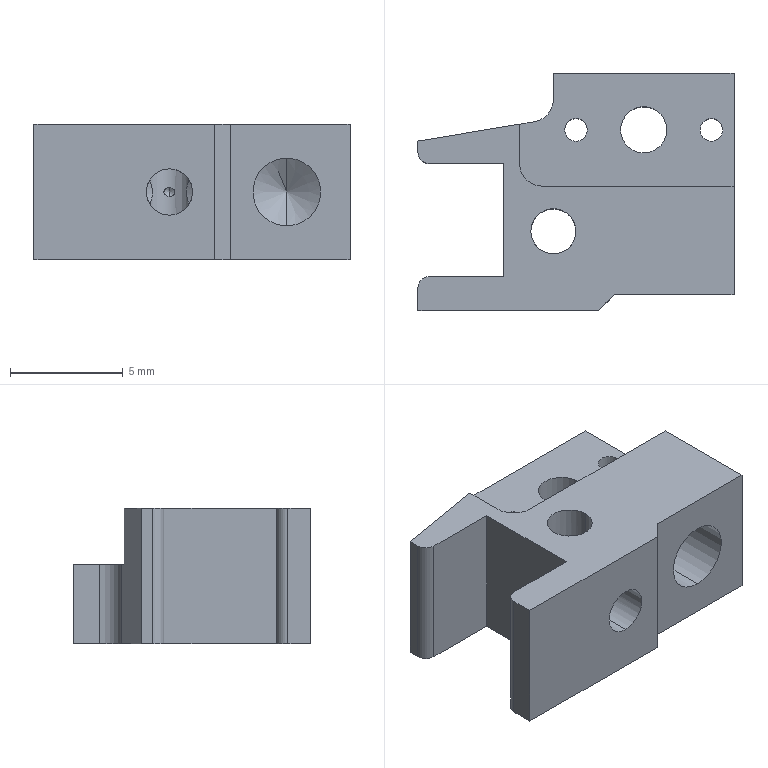Part | SolidWorks | features HoleWzd 5, ICE 4, Fillet 2, Extrusion 1 | 1 solid | 40 faces | box 14 x 10.5 x 6 mm | volume 468.744 mm3 | cylinder 17 | plane 17 | cone 6 | commonest cylinder face diameters 1 x6 2 x5 2.05 x4 3 x2
STEP:
#1=CARTESIAN_POINT('',(-1.,-2.75,1.025));
#2=VERTEX_POINT('',#1);
#3=CARTESIAN_POINT('',(-2.,-1.75,0.225));
#4=VERTEX_POINT('',#3);
#5=CARTESIAN_POINT('',(-1.,-2.75,1.025));
#6=CARTESIAN_POINT('',(-1.149,-2.75,1.025));
#7=CARTESIAN_POINT('',(-1.299,-2.714,0.9901));
#8=CARTESIAN_POINT('',(-1.55,-2.597,0.876));
#9=CARTESIAN_POINT('',(-1.654,-2.516,0.7982));
#10=CARTESIAN_POINT('',(-1.82,-2.336,0.6269));
#11=CARTESIAN_POINT('',(-1.882,-2.236,0.5323));
#12=CARTESIAN_POINT('',(-1.948,-2.074,0.3934));
#13=CARTESIAN_POINT('',(-1.966,-2.018,0.3467));
#14=CARTESIAN_POINT('',(-1.985,-1.925,0.2844));
#15=CARTESIAN_POINT('',(-1.99,-1.893,0.265));
#16=CARTESIAN_POINT('',(-1.998,-1.825,0.235));
#17=CARTESIAN_POINT('',(-2.,-1.787,0.225));
#18=CARTESIAN_POINT('',(-2.,-1.75,0.225));
#19=B_SPLINE_CURVE_WITH_KNOTS('',3,(#5,#6,#7,#8,#9,#10,#11,#12,#13,#14,#15,#16,#17,#18),.UNSPECIFIED.,.F.,.F.,(4,2,2,2,2,2,4),(0.002424,0.002875,0.003325,0.003776,0.004001,0.004114,0.004226),.UNSPECIFIED.);
#20=EDGE_CURVE('',#2,#4,#19,.T.);
#21=ORIENTED_EDGE('',*,*,#20,.F.);
#22=CARTESIAN_POINT('',(-1.,-5.25,1.025));
#23=VERTEX_POINT('',#22);
#24=CARTESIAN_POINT('',(-1.,-5.25,1.025));
#25=DIRECTION('',(0.,-1.,0.));
#26=VECTOR('',#25,1000.);
#27=LINE('',#24,#26);
#28=EDGE_CURVE('',#2,#23,#27,.T.);
#29=ORIENTED_EDGE('',*,*,#28,.T.);
#30=CARTESIAN_POINT('',(-1.,-5.25,-1.025));
#31=VERTEX_POINT('',#30);
#32=CARTESIAN_POINT('',(-1.,-5.25,0.));
#33=DIRECTION('',(0.,-1.,0.));
#34=DIRECTION('',(0.,0.,-1.));
#35=AXIS2_PLACEMENT_3D('',#32,#33,#34);
#36=CIRCLE('',#35,1.025);
#37=EDGE_CURVE('',#23,#31,#36,.T.);
#38=ORIENTED_EDGE('',*,*,#37,.T.);
#39=CARTESIAN_POINT('',(-1.,-2.75,-1.025));
#40=VERTEX_POINT('',#39);
#41=CARTESIAN_POINT('',(-1.,-5.25,-1.025));
#42=DIRECTION('',(0.,-1.,0.));
#43=VECTOR('',#42,1000.);
#44=LINE('',#41,#43);
#45=EDGE_CURVE('',#40,#31,#44,.T.);
#46=ORIENTED_EDGE('',*,*,#45,.F.);
#47=CARTESIAN_POINT('',(-2.,-1.75,-0.225));
#48=VERTEX_POINT('',#47);
#49=CARTESIAN_POINT('',(-2.,-1.75,-0.225));
#50=CARTESIAN_POINT('',(-2.,-1.825,-0.225));
#51=CARTESIAN_POINT('',(-1.991,-1.895,-0.2639));
#52=CARTESIAN_POINT('',(-1.966,-2.018,-0.3468));
#53=CARTESIAN_POINT('',(-1.948,-2.074,-0.3932));
#54=CARTESIAN_POINT('',(-1.882,-2.236,-0.5328));
#55=CARTESIAN_POINT('',(-1.819,-2.336,-0.6275));
#56=CARTESIAN_POINT('',(-1.654,-2.517,-0.7983));
#57=CARTESIAN_POINT('',(-1.55,-2.597,-0.876));
#58=CARTESIAN_POINT('',(-1.36,-2.686,-0.9622));
#59=CARTESIAN_POINT('',(-1.293,-2.709,-0.985));
#60=CARTESIAN_POINT('',(-1.15,-2.741,-1.017));
#61=CARTESIAN_POINT('',(-1.075,-2.75,-1.025));
#62=CARTESIAN_POINT('',(-1.,-2.75,-1.025));
#63=B_SPLINE_CURVE_WITH_KNOTS('',3,(#49,#50,#51,#52,#53,#54,#55,#56,#57,#58,#59,#60,#61,#62),.UNSPECIFIED.,.F.,.F.,(4,2,2,2,2,2,4),(0.0006218,0.0008471,0.001072,0.001523,0.001974,0.002199,0.002424),.UNSPECIFIED.);
#64=EDGE_CURVE('',#48,#40,#63,.T.);
#65=ORIENTED_EDGE('',*,*,#64,.F.);
#66=CARTESIAN_POINT('',(-1.866,-1.25,-0.5483));
#67=VERTEX_POINT('',#66);
#68=CARTESIAN_POINT('',(-1.866,-1.25,-0.5483));
#69=CARTESIAN_POINT('',(-1.907,-1.321,-0.4836));
#70=CARTESIAN_POINT('',(-1.938,-1.395,-0.4176));
#71=CARTESIAN_POINT('',(-1.973,-1.515,-0.3245));
#72=CARTESIAN_POINT('',(-1.982,-1.557,-0.2942));
#73=CARTESIAN_POINT('',(-1.996,-1.647,-0.2444));
#74=CARTESIAN_POINT('',(-2.,-1.698,-0.225));
#75=CARTESIAN_POINT('',(-2.,-1.75,-0.225));
#76=B_SPLINE_CURVE_WITH_KNOTS('',3,(#68,#69,#70,#71,#72,#73,#74,#75),.UNSPECIFIED.,.F.,.F.,(4,2,2,4),(0.,0.0003109,0.0004664,0.0006218),.UNSPECIFIED.);
#77=EDGE_CURVE('',#67,#48,#76,.T.);
#78=ORIENTED_EDGE('',*,*,#77,.F.);
#79=CARTESIAN_POINT('',(-1.866,-1.25,0.5483));
#80=VERTEX_POINT('',#79);
#81=CARTESIAN_POINT('',(-1.,-1.25,0.));
#82=DIRECTION('',(0.,-1.,0.));
#83=DIRECTION('',(0.,0.,-1.));
#84=AXIS2_PLACEMENT_3D('',#81,#82,#83);
#85=CIRCLE('',#84,1.025);
#86=EDGE_CURVE('',#80,#67,#85,.T.);
#87=ORIENTED_EDGE('',*,*,#86,.F.);
#88=CARTESIAN_POINT('',(-2.,-1.75,0.225));
#89=CARTESIAN_POINT('',(-2.,-1.698,0.225));
#90=CARTESIAN_POINT('',(-1.996,-1.647,0.2444));
#91=CARTESIAN_POINT('',(-1.982,-1.556,0.2945));
#92=CARTESIAN_POINT('',(-1.973,-1.515,0.3244));
#93=CARTESIAN_POINT('',(-1.939,-1.395,0.4171));
#94=CARTESIAN_POINT('',(-1.907,-1.321,0.4837));
#95=CARTESIAN_POINT('',(-1.866,-1.25,0.5483));
#96=B_SPLINE_CURVE_WITH_KNOTS('',3,(#88,#89,#90,#91,#92,#93,#94,#95),.UNSPECIFIED.,.F.,.F.,(4,2,2,4),(0.004226,0.004383,0.00454,0.004853),.UNSPECIFIED.);
#97=EDGE_CURVE('',#4,#80,#96,.T.);
#98=ORIENTED_EDGE('',*,*,#97,.F.);
#99=EDGE_LOOP('',(#21,#29,#38,#46,#65,#78,#87,#98));
#100=FACE_OUTER_BOUND('',#99,.T.);
#101=CARTESIAN_POINT('',(-1.,-5.25,0.));
#102=DIRECTION('',(0.,-1.,0.));
#103=DIRECTION('',(0.,0.,-1.));
#104=AXIS2_PLACEMENT_3D('',#101,#102,#103);
#105=CYLINDRICAL_SURFACE('',#104,1.025);
#106=ADVANCED_FACE('',(#100),#105,.F.);
#107=CARTESIAN_POINT('',(-1.,-0.6341,0.));
#108=VERTEX_POINT('',#107);
#109=CARTESIAN_POINT('',(-1.,-0.75,-0.1929));
#110=VERTEX_POINT('',#109);
#111=CARTESIAN_POINT('',(-1.,-1.25,-1.025));
#112=DIRECTION('',(0.,-0.515,-0.8572));
#113=VECTOR('',#112,1000.);
#114=LINE('',#111,#113);
#115=EDGE_CURVE('',#108,#110,#114,.T.);
#116=ORIENTED_EDGE('',*,*,#115,.F.);
#117=CARTESIAN_POINT('',(-1.,-0.75,0.1929));
#118=VERTEX_POINT('',#117);
#119=CARTESIAN_POINT('',(-1.,-1.25,1.025));
#120=DIRECTION('',(0.,-0.515,0.8572));
#121=VECTOR('',#120,1000.);
#122=LINE('',#119,#121);
#123=EDGE_CURVE('',#108,#118,#122,.T.);
#124=ORIENTED_EDGE('',*,*,#123,.T.);
#125=CARTESIAN_POINT('',(-1.,-0.75,-0.1929));
#126=CARTESIAN_POINT('',(-1.057,-0.75,-0.1929));
#127=CARTESIAN_POINT('',(-1.114,-0.7554,-0.1757));
#128=CARTESIAN_POINT('',(-1.207,-0.7704,-0.1091));
#129=CARTESIAN_POINT('',(-1.243,-0.7799,-0.05678));
#130=CARTESIAN_POINT('',(-1.243,-0.7799,0.02858));
#131=CARTESIAN_POINT('',(-1.233,-0.7775,0.0572));
#132=CARTESIAN_POINT('',(-1.203,-0.7708,0.1054));
#133=CARTESIAN_POINT('',(-1.183,-0.7666,0.126));
#134=CARTESIAN_POINT('',(-1.114,-0.7555,0.1753));
#135=CARTESIAN_POINT('',(-1.057,-0.75,0.1929));
#136=CARTESIAN_POINT('',(-1.,-0.75,0.1929));
#137=B_SPLINE_CURVE_WITH_KNOTS('',3,(#125,#126,#127,#128,#129,#130,#131,#132,#133,#134,#135,#136),.UNSPECIFIED.,.F.,.F.,(4,2,2,2,2,4),(0.001171,0.001342,0.001513,0.001599,0.001685,0.001856),.UNSPECIFIED.);
#138=EDGE_CURVE('',#110,#118,#137,.T.);
#139=ORIENTED_EDGE('',*,*,#138,.F.);
#140=EDGE_LOOP('',(#116,#124,#139));
#141=FACE_OUTER_BOUND('',#140,.T.);
#142=CARTESIAN_POINT('',(-1.,-1.25,0.));
#143=DIRECTION('',(0.,-1.,0.));
#144=DIRECTION('',(0.,0.,-1.));
#145=AXIS2_PLACEMENT_3D('',#142,#143,#144);
#146=CONICAL_SURFACE('',#145,1.025,1.03);
#147=ADVANCED_FACE('',(#141),#146,.F.);
#148=CARTESIAN_POINT('',(4.2,-0.55,1.5));
#149=VERTEX_POINT('',#148);
#150=CARTESIAN_POINT('',(4.2,-0.55,-1.5));
#151=VERTEX_POINT('',#150);
#152=CARTESIAN_POINT('',(4.2,-0.55,0.));
#153=DIRECTION('',(0.,-1.,0.));
#154=DIRECTION('',(0.,0.,-1.));
#155=AXIS2_PLACEMENT_3D('',#152,#153,#154);
#156=CIRCLE('',#155,1.5);
#157=EDGE_CURVE('',#149,#151,#156,.T.);
#158=ORIENTED_EDGE('',*,*,#157,.F.);
#159=CARTESIAN_POINT('',(4.2,-4.55,1.5));
#160=VERTEX_POINT('',#159);
#161=CARTESIAN_POINT('',(4.2,-4.55,1.5));
#162=DIRECTION('',(0.,-1.,0.));
#163=VECTOR('',#162,1000.);
#164=LINE('',#161,#163);
#165=EDGE_CURVE('',#149,#160,#164,.T.);
#166=ORIENTED_EDGE('',*,*,#165,.T.);
#167=CARTESIAN_POINT('',(4.2,-4.55,-1.5));
#168=VERTEX_POINT('',#167);
#169=CARTESIAN_POINT('',(4.2,-4.55,0.));
#170=DIRECTION('',(0.,-1.,0.));
#171=DIRECTION('',(0.,0.,-1.));
#172=AXIS2_PLACEMENT_3D('',#169,#170,#171);
#173=CIRCLE('',#172,1.5);
#174=EDGE_CURVE('',#160,#168,#173,.T.);
#175=ORIENTED_EDGE('',*,*,#174,.T.);
#176=CARTESIAN_POINT('',(4.2,-4.55,-1.5));
#177=DIRECTION('',(0.,-1.,0.));
#178=VECTOR('',#177,1000.);
#179=LINE('',#176,#178);
#180=EDGE_CURVE('',#151,#168,#179,.T.);
#181=ORIENTED_EDGE('',*,*,#180,.F.);
#182=EDGE_LOOP('',(#158,#166,#175,#181));
#183=FACE_OUTER_BOUND('',#182,.T.);
#184=CARTESIAN_POINT('',(4.2,-4.55,0.));
#185=DIRECTION('',(0.,-1.,0.));
#186=DIRECTION('',(0.,0.,-1.));
#187=AXIS2_PLACEMENT_3D('',#184,#185,#186);
#188=CYLINDRICAL_SURFACE('',#187,1.5);
#189=ADVANCED_FACE('',(#183),#188,.F.);
#190=CARTESIAN_POINT('',(4.2,0.3513,0.));
#191=VERTEX_POINT('',#190);
#192=CARTESIAN_POINT('',(4.2,-0.55,-1.5));
#193=DIRECTION('',(0.,-0.515,-0.8572));
#194=VECTOR('',#193,1000.);
#195=LINE('',#192,#194);
#196=EDGE_CURVE('',#191,#151,#195,.T.);
#197=ORIENTED_EDGE('',*,*,#196,.F.);
#198=CARTESIAN_POINT('',(4.2,-0.55,1.5));
#199=DIRECTION('',(0.,-0.515,0.8572));
#200=VECTOR('',#199,1000.);
#201=LINE('',#198,#200);
#202=EDGE_CURVE('',#191,#149,#201,.T.);
#203=ORIENTED_EDGE('',*,*,#202,.T.);
#204=ORIENTED_EDGE('',*,*,#157,.T.);
#205=EDGE_LOOP('',(#197,#203,#204));
#206=FACE_OUTER_BOUND('',#205,.T.);
#207=CARTESIAN_POINT('',(4.2,-0.55,0.));
#208=DIRECTION('',(0.,-1.,0.));
#209=DIRECTION('',(0.,0.,-1.));
#210=AXIS2_PLACEMENT_3D('',#207,#208,#209);
#211=CONICAL_SURFACE('',#210,1.5,1.03);
#212=ADVANCED_FACE('',(#206),#211,.F.);
#213=CARTESIAN_POINT('',(-2.,-1.75,-3.));
#214=VERTEX_POINT('',#213);
#215=CARTESIAN_POINT('',(0.,-1.75,-3.));
#216=VERTEX_POINT('',#215);
#217=CARTESIAN_POINT('',(-1.,-1.75,-3.));
#218=DIRECTION('',(0.,0.,1.));
#219=DIRECTION('',(1.,0.,0.));
#220=AXIS2_PLACEMENT_3D('',#217,#218,#219);
#221=CIRCLE('',#220,1.);
#222=EDGE_CURVE('',#214,#216,#221,.T.);
#223=ORIENTED_EDGE('',*,*,#222,.F.);
#224=CARTESIAN_POINT('',(-2.,-1.75,3.));
#225=DIRECTION('',(0.,0.,1.));
#226=VECTOR('',#225,1000.);
#227=LINE('',#224,#226);
#228=EDGE_CURVE('',#214,#48,#227,.T.);
#229=ORIENTED_EDGE('',*,*,#228,.T.);
#230=ORIENTED_EDGE('',*,*,#64,.T.);
#231=CARTESIAN_POINT('',(0.,-1.75,-0.225));
#232=VERTEX_POINT('',#231);
#233=CARTESIAN_POINT('',(-1.,-2.75,-1.025));
#234=CARTESIAN_POINT('',(-0.8509,-2.75,-1.025));
#235=CARTESIAN_POINT('',(-0.7012,-2.714,-0.9901));
#236=CARTESIAN_POINT('',(-0.4503,-2.597,-0.876));
#237=CARTESIAN_POINT('',(-0.346,-2.516,-0.7982));
#238=CARTESIAN_POINT('',(-0.1804,-2.336,-0.6269));
#239=CARTESIAN_POINT('',(-0.1181,-2.236,-0.5323));
#240=CARTESIAN_POINT('',(-0.05212,-2.074,-0.3934));
#241=CARTESIAN_POINT('',(-0.03443,-2.018,-0.3467));
#242=CARTESIAN_POINT('',(-0.01502,-1.925,-0.2844));
#243=CARTESIAN_POINT('',(-0.009736,-1.893,-0.265));
#244=CARTESIAN_POINT('',(-0.002191,-1.825,-0.235));
#245=CARTESIAN_POINT('',(0.,-1.787,-0.225));
#246=CARTESIAN_POINT('',(0.,-1.75,-0.225));
#247=B_SPLINE_CURVE_WITH_KNOTS('',3,(#233,#234,#235,#236,#237,#238,#239,#240,#241,#242,#243,#244,#245,#246),.UNSPECIFIED.,.F.,.F.,(4,2,2,2,2,2,4),(0.002424,0.002875,0.003325,0.003776,0.004001,0.004114,0.004226),.UNSPECIFIED.);
#248=EDGE_CURVE('',#40,#232,#247,.T.);
#249=ORIENTED_EDGE('',*,*,#248,.T.);
#250=CARTESIAN_POINT('',(0.,-1.75,3.));
#251=DIRECTION('',(0.,0.,1.));
#252=VECTOR('',#251,1000.);
#253=LINE('',#250,#252);
#254=EDGE_CURVE('',#216,#232,#253,.T.);
#255=ORIENTED_EDGE('',*,*,#254,.F.);
#256=EDGE_LOOP('',(#223,#229,#230,#249,#255));
#257=FACE_OUTER_BOUND('',#256,.T.);
#258=CARTESIAN_POINT('',(-1.,-1.75,3.));
#259=DIRECTION('',(0.,0.,1.));
#260=DIRECTION('',(1.,0.,0.));
#261=AXIS2_PLACEMENT_3D('',#258,#259,#260);
#262=CYLINDRICAL_SURFACE('',#261,1.);
#263=ADVANCED_FACE('',(#257),#262,.F.);
#264=CARTESIAN_POINT('',(0.,-1.75,0.225));
#265=VERTEX_POINT('',#264);
#266=CARTESIAN_POINT('',(0.,-1.75,0.225));
#267=CARTESIAN_POINT('',(0.,-1.825,0.225));
#268=CARTESIAN_POINT('',(-0.008603,-1.895,0.2639));
#269=CARTESIAN_POINT('',(-0.03449,-2.018,0.3468));
#270=CARTESIAN_POINT('',(-0.05201,-2.074,0.3932));
#271=CARTESIAN_POINT('',(-0.1183,-2.236,0.5328));
#272=CARTESIAN_POINT('',(-0.1808,-2.336,0.6275));
#273=CARTESIAN_POINT('',(-0.3462,-2.517,0.7983));
#274=CARTESIAN_POINT('',(-0.45,-2.597,0.876));
#275=CARTESIAN_POINT('',(-0.6399,-2.686,0.9622));
#276=CARTESIAN_POINT('',(-0.7072,-2.709,0.985));
#277=CARTESIAN_POINT('',(-0.8503,-2.741,1.017));
#278=CARTESIAN_POINT('',(-0.9254,-2.75,1.025));
#279=CARTESIAN_POINT('',(-1.,-2.75,1.025));
#280=B_SPLINE_CURVE_WITH_KNOTS('',3,(#266,#267,#268,#269,#270,#271,#272,#273,#274,#275,#276,#277,#278,#279),.UNSPECIFIED.,.F.,.F.,(4,2,2,2,2,2,4),(0.0006218,0.0008471,0.001072,0.001523,0.001974,0.002199,0.002424),.UNSPECIFIED.);
#281=EDGE_CURVE('',#265,#2,#280,.T.);
#282=ORIENTED_EDGE('',*,*,#281,.T.);
#283=ORIENTED_EDGE('',*,*,#20,.T.);
#284=CARTESIAN_POINT('',(-2.,-1.75,3.));
#285=VERTEX_POINT('',#284);
#286=CARTESIAN_POINT('',(-2.,-1.75,3.));
#287=DIRECTION('',(0.,0.,1.));
#288=VECTOR('',#287,1000.);
#289=LINE('',#286,#288);
#290=EDGE_CURVE('',#4,#285,#289,.T.);
#291=ORIENTED_EDGE('',*,*,#290,.T.);
#292=CARTESIAN_POINT('',(0.,-1.75,3.));
#293=VERTEX_POINT('',#292);
#294=CARTESIAN_POINT('',(-1.,-1.75,3.));
#295=DIRECTION('',(0.,0.,1.));
#296=DIRECTION('',(1.,0.,0.));
#297=AXIS2_PLACEMENT_3D('',#294,#295,#296);
#298=CIRCLE('',#297,1.);
#299=EDGE_CURVE('',#285,#293,#298,.T.);
#300=ORIENTED_EDGE('',*,*,#299,.T.);
#301=CARTESIAN_POINT('',(0.,-1.75,3.));
#302=DIRECTION('',(0.,0.,1.));
#303=VECTOR('',#302,1000.);
#304=LINE('',#301,#303);
#305=EDGE_CURVE('',#265,#293,#304,.T.);
#306=ORIENTED_EDGE('',*,*,#305,.F.);
#307=EDGE_LOOP('',(#282,#283,#291,#300,#306));
#308=FACE_OUTER_BOUND('',#307,.T.);
#309=CARTESIAN_POINT('',(-1.,-1.75,3.));
#310=DIRECTION('',(0.,0.,1.));
#311=DIRECTION('',(1.,0.,0.));
#312=AXIS2_PLACEMENT_3D('',#309,#310,#311);
#313=CYLINDRICAL_SURFACE('',#312,1.);
#314=ADVANCED_FACE('',(#308),#313,.F.);
#315=CARTESIAN_POINT('',(-0.5,2.75,-3.));
#316=VERTEX_POINT('',#315);
#317=CARTESIAN_POINT('',(0.5,2.75,-3.));
#318=VERTEX_POINT('',#317);
#319=CARTESIAN_POINT('',(0.,2.75,-3.));
#320=DIRECTION('',(0.,0.,1.));
#321=DIRECTION('',(1.,0.,0.));
#322=AXIS2_PLACEMENT_3D('',#319,#320,#321);
#323=CIRCLE('',#322,0.5);
#324=EDGE_CURVE('',#316,#318,#323,.T.);
#325=ORIENTED_EDGE('',*,*,#324,.F.);
#326=CARTESIAN_POINT('',(-0.5,2.75,0.5));
#327=VERTEX_POINT('',#326);
#328=CARTESIAN_POINT('',(-0.5,2.75,0.5));
#329=DIRECTION('',(0.,0.,1.));
#330=VECTOR('',#329,1000.);
#331=LINE('',#328,#330);
#332=EDGE_CURVE('',#316,#327,#331,.T.);
#333=ORIENTED_EDGE('',*,*,#332,.T.);
#334=CARTESIAN_POINT('',(0.5,2.75,0.5));
#335=VERTEX_POINT('',#334);
#336=CARTESIAN_POINT('',(0.,2.75,0.5));
#337=DIRECTION('',(0.,0.,1.));
#338=DIRECTION('',(1.,0.,0.));
#339=AXIS2_PLACEMENT_3D('',#336,#337,#338);
#340=CIRCLE('',#339,0.5);
#341=EDGE_CURVE('',#327,#335,#340,.T.);
#342=ORIENTED_EDGE('',*,*,#341,.T.);
#343=CARTESIAN_POINT('',(0.5,2.75,0.5));
#344=DIRECTION('',(0.,0.,1.));
#345=VECTOR('',#344,1000.);
#346=LINE('',#343,#345);
#347=EDGE_CURVE('',#318,#335,#346,.T.);
#348=ORIENTED_EDGE('',*,*,#347,.F.);
#349=EDGE_LOOP('',(#325,#333,#342,#348));
#350=FACE_OUTER_BOUND('',#349,.T.);
#351=CARTESIAN_POINT('',(0.,2.75,0.5));
#352=DIRECTION('',(0.,0.,1.));
#353=DIRECTION('',(1.,0.,0.));
#354=AXIS2_PLACEMENT_3D('',#351,#352,#353);
#355=CYLINDRICAL_SURFACE('',#354,0.5);
#356=ADVANCED_FACE('',(#350),#355,.F.);
#357=CARTESIAN_POINT('',(5.5,2.75,-3.));
#358=VERTEX_POINT('',#357);
#359=CARTESIAN_POINT('',(6.5,2.75,-3.));
#360=VERTEX_POINT('',#359);
#361=CARTESIAN_POINT('',(6.,2.75,-3.));
#362=DIRECTION('',(0.,0.,1.));
#363=DIRECTION('',(1.,0.,0.));
#364=AXIS2_PLACEMENT_3D('',#361,#362,#363);
#365=CIRCLE('',#364,0.5);
#366=EDGE_CURVE('',#358,#360,#365,.T.);
#367=ORIENTED_EDGE('',*,*,#366,.F.);
#368=CARTESIAN_POINT('',(5.5,2.75,0.5));
#369=VERTEX_POINT('',#368);
#370=CARTESIAN_POINT('',(5.5,2.75,0.5));
#371=DIRECTION('',(0.,0.,1.));
#372=VECTOR('',#371,1000.);
#373=LINE('',#370,#372);
#374=EDGE_CURVE('',#358,#369,#373,.T.);
#375=ORIENTED_EDGE('',*,*,#374,.T.);
#376=CARTESIAN_POINT('',(6.5,2.75,0.5));
#377=VERTEX_POINT('',#376);
#378=CARTESIAN_POINT('',(6.,2.75,0.5));
#379=DIRECTION('',(0.,0.,1.));
#380=DIRECTION('',(1.,0.,0.));
#381=AXIS2_PLACEMENT_3D('',#378,#379,#380);
#382=CIRCLE('',#381,0.5);
#383=EDGE_CURVE('',#369,#377,#382,.T.);
#384=ORIENTED_EDGE('',*,*,#383,.T.);
#385=CARTESIAN_POINT('',(6.5,2.75,0.5));
#386=DIRECTION('',(0.,0.,1.));
#387=VECTOR('',#386,1000.);
#388=LINE('',#385,#387);
#389=EDGE_CURVE('',#360,#377,#388,.T.);
#390=ORIENTED_EDGE('',*,*,#389,.F.);
#391=EDGE_LOOP('',(#367,#375,#384,#390));
#392=FACE_OUTER_BOUND('',#391,.T.);
#393=CARTESIAN_POINT('',(6.,2.75,0.5));
#394=DIRECTION('',(0.,0.,1.));
#395=DIRECTION('',(1.,0.,0.));
#396=AXIS2_PLACEMENT_3D('',#393,#394,#395);
#397=CYLINDRICAL_SURFACE('',#396,0.5);
#398=ADVANCED_FACE('',(#392),#397,.F.);
#399=CARTESIAN_POINT('',(1.975,2.75,-3.));
#400=VERTEX_POINT('',#399);
#401=CARTESIAN_POINT('',(4.025,2.75,-3.));
#402=VERTEX_POINT('',#401);
#403=CARTESIAN_POINT('',(3.,2.75,-3.));
#404=DIRECTION('',(0.,0.,1.));
#405=DIRECTION('',(1.,0.,0.));
#406=AXIS2_PLACEMENT_3D('',#403,#404,#405);
#407=CIRCLE('',#406,1.025);
#408=EDGE_CURVE('',#400,#402,#407,.T.);
#409=ORIENTED_EDGE('',*,*,#408,.F.);
#410=CARTESIAN_POINT('',(1.975,2.75,0.5));
#411=VERTEX_POINT('',#410);
#412=CARTESIAN_POINT('',(1.975,2.75,0.5));
#413=DIRECTION('',(0.,0.,1.));
#414=VECTOR('',#413,1000.);
#415=LINE('',#412,#414);
#416=EDGE_CURVE('',#400,#411,#415,.T.);
#417=ORIENTED_EDGE('',*,*,#416,.T.);
#418=CARTESIAN_POINT('',(4.025,2.75,0.5));
#419=VERTEX_POINT('',#418);
#420=CARTESIAN_POINT('',(3.,2.75,0.5));
#421=DIRECTION('',(0.,0.,1.));
#422=DIRECTION('',(1.,0.,0.));
#423=AXIS2_PLACEMENT_3D('',#420,#421,#422);
#424=CIRCLE('',#423,1.025);
#425=EDGE_CURVE('',#411,#419,#424,.T.);
#426=ORIENTED_EDGE('',*,*,#425,.T.);
#427=CARTESIAN_POINT('',(4.025,2.75,0.5));
#428=DIRECTION('',(0.,0.,1.));
#429=VECTOR('',#428,1000.);
#430=LINE('',#427,#429);
#431=EDGE_CURVE('',#402,#419,#430,.T.);
#432=ORIENTED_EDGE('',*,*,#431,.F.);
#433=EDGE_LOOP('',(#409,#417,#426,#432));
#434=FACE_OUTER_BOUND('',#433,.T.);
#435=CARTESIAN_POINT('',(3.,2.75,0.5));
#436=DIRECTION('',(0.,0.,1.));
#437=DIRECTION('',(1.,0.,0.));
#438=AXIS2_PLACEMENT_3D('',#435,#436,#437);
#439=CYLINDRICAL_SURFACE('',#438,1.025);
#440=ADVANCED_FACE('',(#434),#439,.F.);
#441=CARTESIAN_POINT('',(-7.,2.25,-3.));
#442=VERTEX_POINT('',#441);
#443=CARTESIAN_POINT('',(-7.,1.75,-3.));
#444=VERTEX_POINT('',#443);
#445=CARTESIAN_POINT('',(-7.,5.25,-3.));
#446=DIRECTION('',(0.,-1.,0.));
#447=VECTOR('',#446,1000.);
#448=LINE('',#445,#447);
#449=EDGE_CURVE('',#442,#444,#448,.T.);
#450=ORIENTED_EDGE('',*,*,#449,.T.);
#451=CARTESIAN_POINT('',(-7.,1.75,3.));
#452=VERTEX_POINT('',#451);
#453=CARTESIAN_POINT('',(-7.,1.75,3.));
#454=DIRECTION('',(0.,0.,1.));
#455=VECTOR('',#454,1000.);
#456=LINE('',#453,#455);
#457=EDGE_CURVE('',#444,#452,#456,.T.);
#458=ORIENTED_EDGE('',*,*,#457,.T.);
#459=CARTESIAN_POINT('',(-7.,2.25,3.));
#460=VERTEX_POINT('',#459);
#461=CARTESIAN_POINT('',(-7.,5.25,3.));
#462=DIRECTION('',(0.,-1.,0.));
#463=VECTOR('',#462,1000.);
#464=LINE('',#461,#463);
#465=EDGE_CURVE('',#460,#452,#464,.T.);
#466=ORIENTED_EDGE('',*,*,#465,.F.);
#467=CARTESIAN_POINT('',(-7.,2.25,-3.));
#468=DIRECTION('',(0.,0.,1.));
#469=VECTOR('',#468,1000.);
#470=LINE('',#467,#469);
#471=EDGE_CURVE('',#442,#460,#470,.T.);
#472=ORIENTED_EDGE('',*,*,#471,.F.);
#473=EDGE_LOOP('',(#450,#458,#466,#472));
#474=FACE_OUTER_BOUND('',#473,.T.);
#475=CARTESIAN_POINT('',(-7.,5.25,3.));
#476=DIRECTION('',(1.,0.,0.));
#477=DIRECTION('',(0.,1.,0.));
#478=AXIS2_PLACEMENT_3D('',#475,#476,#477);
#479=PLANE('',#478);
#480=ADVANCED_FACE('',(#474),#479,.F.);
#481=CARTESIAN_POINT('',(7.,-4.55,3.));
#482=VERTEX_POINT('',#481);
#483=CARTESIAN_POINT('',(7.,0.25,3.));
#484=VERTEX_POINT('',#483);
#485=CARTESIAN_POINT('',(7.,5.25,3.));
#486=DIRECTION('',(0.,1.,0.));
#487=VECTOR('',#486,1000.);
#488=LINE('',#485,#487);
#489=EDGE_CURVE('',#482,#484,#488,.T.);
#490=ORIENTED_EDGE('',*,*,#489,.F.);
#491=CARTESIAN_POINT('',(7.,-4.55,-3.));
#492=VERTEX_POINT('',#491);
#493=CARTESIAN_POINT('',(7.,-4.55,-3.));
#494=DIRECTION('',(0.,0.,1.));
#495=VECTOR('',#494,1000.);
#496=LINE('',#493,#495);
#497=EDGE_CURVE('',#492,#482,#496,.T.);
#498=ORIENTED_EDGE('',*,*,#497,.F.);
#499=CARTESIAN_POINT('',(7.,5.25,-3.));
#500=VERTEX_POINT('',#499);
#501=CARTESIAN_POINT('',(7.,5.25,-3.));
#502=DIRECTION('',(0.,1.,0.));
#503=VECTOR('',#502,1000.);
#504=LINE('',#501,#503);
#505=EDGE_CURVE('',#492,#500,#504,.T.);
#506=ORIENTED_EDGE('',*,*,#505,.T.);
#507=CARTESIAN_POINT('',(7.,5.25,0.5));
#508=VERTEX_POINT('',#507);
#509=CARTESIAN_POINT('',(7.,5.25,3.));
#510=DIRECTION('',(0.,0.,-1.));
#511=VECTOR('',#510,1000.);
#512=LINE('',#509,#511);
#513=EDGE_CURVE('',#508,#500,#512,.T.);
#514=ORIENTED_EDGE('',*,*,#513,.F.);
#515=CARTESIAN_POINT('',(7.,0.25,0.5));
#516=VERTEX_POINT('',#515);
#517=CARTESIAN_POINT('',(7.,5.25,0.5));
#518=DIRECTION('',(0.,1.,0.));
#519=VECTOR('',#518,1000.);
#520=LINE('',#517,#519);
#521=EDGE_CURVE('',#516,#508,#520,.T.);
#522=ORIENTED_EDGE('',*,*,#521,.F.);
#523=CARTESIAN_POINT('',(7.,0.25,0.5));
#524=DIRECTION('',(0.,0.,1.));
#525=VECTOR('',#524,1000.);
#526=LINE('',#523,#525);
#527=EDGE_CURVE('',#516,#484,#526,.T.);
#528=ORIENTED_EDGE('',*,*,#527,.T.);
#529=EDGE_LOOP('',(#490,#498,#506,#514,#522,#528));
#530=FACE_OUTER_BOUND('',#529,.T.);
#531=CARTESIAN_POINT('',(7.,5.25,3.));
#532=DIRECTION('',(-1.,0.,0.));
#533=DIRECTION('',(0.,-1.,0.));
#534=AXIS2_PLACEMENT_3D('',#531,#532,#533);
#535=PLANE('',#534);
#536=ADVANCED_FACE('',(#530),#535,.F.);
#537=CARTESIAN_POINT('',(-1.,5.25,-3.));
#538=VERTEX_POINT('',#537);
#539=CARTESIAN_POINT('',(-7.,5.25,-3.));
#540=DIRECTION('',(-1.,0.,0.));
#541=VECTOR('',#540,1000.);
#542=LINE('',#539,#541);
#543=EDGE_CURVE('',#500,#538,#542,.T.);
#544=ORIENTED_EDGE('',*,*,#543,.T.);
#545=CARTESIAN_POINT('',(-1.,5.25,0.5));
#546=VERTEX_POINT('',#545);
#547=CARTESIAN_POINT('',(-1.,5.25,-3.));
#548=DIRECTION('',(0.,0.,1.));
#549=VECTOR('',#548,1000.);
#550=LINE('',#547,#549);
#551=EDGE_CURVE('',#538,#546,#550,.T.);
#552=ORIENTED_EDGE('',*,*,#551,.T.);
#553=CARTESIAN_POINT('',(7.,5.25,0.5));
#554=DIRECTION('',(-1.,0.,0.));
#555=VECTOR('',#554,1000.);
#556=LINE('',#553,#555);
#557=EDGE_CURVE('',#508,#546,#556,.T.);
#558=ORIENTED_EDGE('',*,*,#557,.F.);
#559=ORIENTED_EDGE('',*,*,#513,.T.);
#560=EDGE_LOOP('',(#544,#552,#558,#559));
#561=FACE_OUTER_BOUND('',#560,.T.);
#562=CARTESIAN_POINT('',(-7.,5.25,3.));
#563=DIRECTION('',(0.,-1.,0.));
#564=DIRECTION('',(0.,0.,-1.));
#565=AXIS2_PLACEMENT_3D('',#562,#563,#564);
#566=PLANE('',#565);
#567=ADVANCED_FACE('',(#561),#566,.F.);
#568=CARTESIAN_POINT('',(-7.,-4.25,3.));
#569=VERTEX_POINT('',#568);
#570=CARTESIAN_POINT('',(-7.,-5.25,3.));
#571=VERTEX_POINT('',#570);
#572=CARTESIAN_POINT('',(-7.,5.25,3.));
#573=DIRECTION('',(0.,-1.,0.));
#574=VECTOR('',#573,1000.);
#575=LINE('',#572,#574);
#576=EDGE_CURVE('',#569,#571,#575,.T.);
#577=ORIENTED_EDGE('',*,*,#576,.F.);
#578=CARTESIAN_POINT('',(-7.,-4.25,-3.));
#579=VERTEX_POINT('',#578);
#580=CARTESIAN_POINT('',(-7.,-4.25,3.));
#581=DIRECTION('',(0.,0.,-1.));
#582=VECTOR('',#581,1000.);
#583=LINE('',#580,#582);
#584=EDGE_CURVE('',#569,#579,#583,.T.);
#585=ORIENTED_EDGE('',*,*,#584,.T.);
#586=CARTESIAN_POINT('',(-7.,-5.25,-3.));
#587=VERTEX_POINT('',#586);
#588=CARTESIAN_POINT('',(-7.,5.25,-3.));
#589=DIRECTION('',(0.,-1.,0.));
#590=VECTOR('',#589,1000.);
#591=LINE('',#588,#590);
#592=EDGE_CURVE('',#579,#587,#591,.T.);
#593=ORIENTED_EDGE('',*,*,#592,.T.);
#594=CARTESIAN_POINT('',(-7.,-5.25,3.));
#595=DIRECTION('',(0.,0.,-1.));
#596=VECTOR('',#595,1000.);
#597=LINE('',#594,#596);
#598=EDGE_CURVE('',#571,#587,#597,.T.);
#599=ORIENTED_EDGE('',*,*,#598,.F.);
#600=EDGE_LOOP('',(#577,#585,#593,#599));
#601=FACE_OUTER_BOUND('',#600,.T.);
#602=CARTESIAN_POINT('',(-7.,5.25,3.));
#603=DIRECTION('',(1.,0.,0.));
#604=DIRECTION('',(0.,1.,0.));
#605=AXIS2_PLACEMENT_3D('',#602,#603,#604);
#606=PLANE('',#605);
#607=ADVANCED_FACE('',(#601),#606,.F.);
#608=CARTESIAN_POINT('',(-1.,-5.25,0.));
#609=DIRECTION('',(0.,-1.,0.));
#610=DIRECTION('',(0.,0.,-1.));
#611=AXIS2_PLACEMENT_3D('',#608,#609,#610);
#612=CIRCLE('',#611,1.025);
#613=EDGE_CURVE('',#31,#23,#612,.T.);
#614=ORIENTED_EDGE('',*,*,#613,.F.);
#615=ORIENTED_EDGE('',*,*,#37,.F.);
#616=EDGE_LOOP('',(#614,#615));
#617=FACE_BOUND('',#616,.T.);
#618=CARTESIAN_POINT('',(1.,-5.25,-3.));
#619=VERTEX_POINT('',#618);
#620=CARTESIAN_POINT('',(-7.,-5.25,-3.));
#621=DIRECTION('',(1.,0.,0.));
#622=VECTOR('',#621,1000.);
#623=LINE('',#620,#622);
#624=EDGE_CURVE('',#587,#619,#623,.T.);
#625=ORIENTED_EDGE('',*,*,#624,.T.);
#626=CARTESIAN_POINT('',(1.,-5.25,3.));
#627=VERTEX_POINT('',#626);
#628=CARTESIAN_POINT('',(1.,-5.25,-3.));
#629=DIRECTION('',(0.,0.,1.));
#630=VECTOR('',#629,1000.);
#631=LINE('',#628,#630);
#632=EDGE_CURVE('',#619,#627,#631,.T.);
#633=ORIENTED_EDGE('',*,*,#632,.T.);
#634=CARTESIAN_POINT('',(-7.,-5.25,3.));
#635=DIRECTION('',(1.,0.,0.));
#636=VECTOR('',#635,1000.);
#637=LINE('',#634,#636);
#638=EDGE_CURVE('',#571,#627,#637,.T.);
#639=ORIENTED_EDGE('',*,*,#638,.F.);
#640=ORIENTED_EDGE('',*,*,#598,.T.);
#641=EDGE_LOOP('',(#625,#633,#639,#640));
#642=FACE_OUTER_BOUND('',#641,.T.);
#643=CARTESIAN_POINT('',(-7.,-5.25,3.));
#644=DIRECTION('',(0.,1.,0.));
#645=DIRECTION('',(0.,0.,1.));
#646=AXIS2_PLACEMENT_3D('',#643,#644,#645);
#647=PLANE('',#646);
#648=ADVANCED_FACE('',(#617,#642),#647,.F.);
#649=ORIENTED_EDGE('',*,*,#465,.T.);
#650=CARTESIAN_POINT('',(-6.5,1.25,3.));
#651=VERTEX_POINT('',#650);
#652=CARTESIAN_POINT('',(-6.5,1.75,3.));
#653=DIRECTION('',(0.,0.,1.));
#654=DIRECTION('',(1.,0.,0.));
#655=AXIS2_PLACEMENT_3D('',#652,#653,#654);
#656=CIRCLE('',#655,0.5);
#657=EDGE_CURVE('',#452,#651,#656,.T.);
#658=ORIENTED_EDGE('',*,*,#657,.T.);
#659=CARTESIAN_POINT('',(-3.2,1.25,3.));
#660=VERTEX_POINT('',#659);
#661=CARTESIAN_POINT('',(-7.,1.25,3.));
#662=DIRECTION('',(-1.,0.,0.));
#663=VECTOR('',#662,1000.);
#664=LINE('',#661,#663);
#665=EDGE_CURVE('',#660,#651,#664,.T.);
#666=ORIENTED_EDGE('',*,*,#665,.F.);
#667=CARTESIAN_POINT('',(-3.2,-3.75,3.));
#668=VERTEX_POINT('',#667);
#669=CARTESIAN_POINT('',(-3.2,-3.75,3.));
#670=DIRECTION('',(0.,1.,0.));
#671=VECTOR('',#670,1000.);
#672=LINE('',#669,#671);
#673=EDGE_CURVE('',#668,#660,#672,.T.);
#674=ORIENTED_EDGE('',*,*,#673,.F.);
#675=CARTESIAN_POINT('',(-6.5,-3.75,3.));
#676=VERTEX_POINT('',#675);
#677=CARTESIAN_POINT('',(-7.,-3.75,3.));
#678=DIRECTION('',(1.,0.,0.));
#679=VECTOR('',#678,1000.);
#680=LINE('',#677,#679);
#681=EDGE_CURVE('',#676,#668,#680,.T.);
#682=ORIENTED_EDGE('',*,*,#681,.F.);
#683=CARTESIAN_POINT('',(-6.5,-4.25,3.));
#684=DIRECTION('',(0.,0.,1.));
#685=DIRECTION('',(1.,0.,0.));
#686=AXIS2_PLACEMENT_3D('',#683,#684,#685);
#687=CIRCLE('',#686,0.5);
#688=EDGE_CURVE('',#676,#569,#687,.T.);
#689=ORIENTED_EDGE('',*,*,#688,.T.);
#690=ORIENTED_EDGE('',*,*,#576,.T.);
#691=ORIENTED_EDGE('',*,*,#638,.T.);
#692=CARTESIAN_POINT('',(1.7,-4.55,3.));
#693=VERTEX_POINT('',#692);
#694=CARTESIAN_POINT('',(1.,-5.25,3.));
#695=DIRECTION('',(-0.7071,-0.7071,0.));
#696=VECTOR('',#695,1000.);
#697=LINE('',#694,#696);
#698=EDGE_CURVE('',#693,#627,#697,.T.);
#699=ORIENTED_EDGE('',*,*,#698,.F.);
#700=CARTESIAN_POINT('',(1.7,-4.55,3.));
#701=DIRECTION('',(-1.,0.,0.));
#702=VECTOR('',#701,1000.);
#703=LINE('',#700,#702);
#704=EDGE_CURVE('',#482,#693,#703,.T.);
#705=ORIENTED_EDGE('',*,*,#704,.F.);
#706=ORIENTED_EDGE('',*,*,#489,.T.);
#707=CARTESIAN_POINT('',(-1.5,0.25,3.));
#708=VERTEX_POINT('',#707);
#709=CARTESIAN_POINT('',(7.,0.25,3.));
#710=DIRECTION('',(1.,0.,0.));
#711=VECTOR('',#710,1000.);
#712=LINE('',#709,#711);
#713=EDGE_CURVE('',#708,#484,#712,.T.);
#714=ORIENTED_EDGE('',*,*,#713,.F.);
#715=CARTESIAN_POINT('',(-2.5,1.25,3.));
#716=VERTEX_POINT('',#715);
#717=CARTESIAN_POINT('',(-1.5,1.25,3.));
#718=DIRECTION('',(0.,0.,-1.));
#719=DIRECTION('',(1.,0.,0.));
#720=AXIS2_PLACEMENT_3D('',#717,#718,#719);
#721=CIRCLE('',#720,1.);
#722=EDGE_CURVE('',#708,#716,#721,.T.);
#723=ORIENTED_EDGE('',*,*,#722,.T.);
#724=CARTESIAN_POINT('',(-2.5,3.,3.));
#725=VERTEX_POINT('',#724);
#726=CARTESIAN_POINT('',(-2.5,5.25,3.));
#727=DIRECTION('',(0.,-1.,0.));
#728=VECTOR('',#727,1000.);
#729=LINE('',#726,#728);
#730=EDGE_CURVE('',#725,#716,#729,.T.);
#731=ORIENTED_EDGE('',*,*,#730,.F.);
#732=CARTESIAN_POINT('',(-1.,3.25,3.));
#733=DIRECTION('',(0.9864,0.1644,0.));
#734=VECTOR('',#733,1000.);
#735=LINE('',#732,#734);
#736=EDGE_CURVE('',#460,#725,#735,.T.);
#737=ORIENTED_EDGE('',*,*,#736,.F.);
#738=EDGE_LOOP('',(#649,#658,#666,#674,#682,#689,#690,#691,#699,#705,#706,#714,#723,#731,#737));
#739=FACE_OUTER_BOUND('',#738,.T.);
#740=CARTESIAN_POINT('',(-1.,-1.75,3.));
#741=DIRECTION('',(0.,0.,1.));
#742=DIRECTION('',(1.,0.,0.));
#743=AXIS2_PLACEMENT_3D('',#740,#741,#742);
#744=CIRCLE('',#743,1.);
#745=EDGE_CURVE('',#293,#285,#744,.T.);
#746=ORIENTED_EDGE('',*,*,#745,.F.);
#747=ORIENTED_EDGE('',*,*,#299,.F.);
#748=EDGE_LOOP('',(#746,#747));
#749=FACE_BOUND('',#748,.T.);
#750=CARTESIAN_POINT('',(0.,0.,3.));
#751=DIRECTION('',(0.,0.,1.));
#752=DIRECTION('',(1.,0.,0.));
#753=AXIS2_PLACEMENT_3D('',#750,#751,#752);
#754=PLANE('',#753);
#755=ADVANCED_FACE('',(#739,#749),#754,.T.);
#756=CARTESIAN_POINT('',(-1.,-1.75,-3.));
#757=DIRECTION('',(0.,0.,1.));
#758=DIRECTION('',(1.,0.,0.));
#759=AXIS2_PLACEMENT_3D('',#756,#757,#758);
#760=CIRCLE('',#759,1.);
#761=EDGE_CURVE('',#216,#214,#760,.T.);
#762=ORIENTED_EDGE('',*,*,#761,.T.);
#763=ORIENTED_EDGE('',*,*,#222,.T.);
#764=EDGE_LOOP('',(#762,#763));
#765=FACE_BOUND('',#764,.T.);
#766=CARTESIAN_POINT('',(0.,2.75,-3.));
#767=DIRECTION('',(0.,0.,1.));
#768=DIRECTION('',(1.,0.,0.));
#769=AXIS2_PLACEMENT_3D('',#766,#767,#768);
#770=CIRCLE('',#769,0.5);
#771=EDGE_CURVE('',#318,#316,#770,.T.);
#772=ORIENTED_EDGE('',*,*,#771,.T.);
#773=ORIENTED_EDGE('',*,*,#324,.T.);
#774=EDGE_LOOP('',(#772,#773));
#775=FACE_BOUND('',#774,.T.);
#776=CARTESIAN_POINT('',(6.,2.75,-3.));
#777=DIRECTION('',(0.,0.,1.));
#778=DIRECTION('',(1.,0.,0.));
#779=AXIS2_PLACEMENT_3D('',#776,#777,#778);
#780=CIRCLE('',#779,0.5);
#781=EDGE_CURVE('',#360,#358,#780,.T.);
#782=ORIENTED_EDGE('',*,*,#781,.T.);
#783=ORIENTED_EDGE('',*,*,#366,.T.);
#784=EDGE_LOOP('',(#782,#783));
#785=FACE_BOUND('',#784,.T.);
#786=CARTESIAN_POINT('',(3.,2.75,-3.));
#787=DIRECTION('',(0.,0.,1.));
#788=DIRECTION('',(1.,0.,0.));
#789=AXIS2_PLACEMENT_3D('',#786,#787,#788);
#790=CIRCLE('',#789,1.025);
#791=EDGE_CURVE('',#402,#400,#790,.T.);
#792=ORIENTED_EDGE('',*,*,#791,.T.);
#793=ORIENTED_EDGE('',*,*,#408,.T.);
#794=EDGE_LOOP('',(#792,#793));
#795=FACE_BOUND('',#794,.T.);
#796=CARTESIAN_POINT('',(-3.2,1.25,-3.));
#797=VERTEX_POINT('',#796);
#798=CARTESIAN_POINT('',(-6.5,1.25,-3.));
#799=VERTEX_POINT('',#798);
#800=CARTESIAN_POINT('',(-7.,1.25,-3.));
#801=DIRECTION('',(-1.,0.,0.));
#802=VECTOR('',#801,1000.);
#803=LINE('',#800,#802);
#804=EDGE_CURVE('',#797,#799,#803,.T.);
#805=ORIENTED_EDGE('',*,*,#804,.T.);
#806=CARTESIAN_POINT('',(-6.5,1.75,-3.));
#807=DIRECTION('',(0.,0.,-1.));
#808=DIRECTION('',(1.,0.,0.));
#809=AXIS2_PLACEMENT_3D('',#806,#807,#808);
#810=CIRCLE('',#809,0.5);
#811=EDGE_CURVE('',#799,#444,#810,.T.);
#812=ORIENTED_EDGE('',*,*,#811,.T.);
#813=ORIENTED_EDGE('',*,*,#449,.F.);
#814=CARTESIAN_POINT('',(-1.836,3.111,-3.));
#815=VERTEX_POINT('',#814);
#816=CARTESIAN_POINT('',(-1.,3.25,-3.));
#817=DIRECTION('',(0.9864,0.1644,0.));
#818=VECTOR('',#817,1000.);
#819=LINE('',#816,#818);
#820=EDGE_CURVE('',#442,#815,#819,.T.);
#821=ORIENTED_EDGE('',*,*,#820,.T.);
#822=CARTESIAN_POINT('',(-1.,4.097,-3.));
#823=VERTEX_POINT('',#822);
#824=CARTESIAN_POINT('',(-2.,4.097,-3.));
#825=DIRECTION('',(0.,0.,1.));
#826=DIRECTION('',(1.,0.,0.));
#827=AXIS2_PLACEMENT_3D('',#824,#825,#826);
#828=CIRCLE('',#827,1.);
#829=EDGE_CURVE('',#815,#823,#828,.T.);
#830=ORIENTED_EDGE('',*,*,#829,.T.);
#831=CARTESIAN_POINT('',(-1.,5.25,-3.));
#832=DIRECTION('',(0.,1.,0.));
#833=VECTOR('',#832,1000.);
#834=LINE('',#831,#833);
#835=EDGE_CURVE('',#823,#538,#834,.T.);
#836=ORIENTED_EDGE('',*,*,#835,.T.);
#837=ORIENTED_EDGE('',*,*,#543,.F.);
#838=ORIENTED_EDGE('',*,*,#505,.F.);
#839=CARTESIAN_POINT('',(1.7,-4.55,-3.));
#840=VERTEX_POINT('',#839);
#841=CARTESIAN_POINT('',(1.7,-4.55,-3.));
#842=DIRECTION('',(-1.,0.,0.));
#843=VECTOR('',#842,1000.);
#844=LINE('',#841,#843);
#845=EDGE_CURVE('',#492,#840,#844,.T.);
#846=ORIENTED_EDGE('',*,*,#845,.T.);
#847=CARTESIAN_POINT('',(1.,-5.25,-3.));
#848=DIRECTION('',(-0.7071,-0.7071,0.));
#849=VECTOR('',#848,1000.);
#850=LINE('',#847,#849);
#851=EDGE_CURVE('',#840,#619,#850,.T.);
#852=ORIENTED_EDGE('',*,*,#851,.T.);
#853=ORIENTED_EDGE('',*,*,#624,.F.);
#854=ORIENTED_EDGE('',*,*,#592,.F.);
#855=CARTESIAN_POINT('',(-6.5,-3.75,-3.));
#856=VERTEX_POINT('',#855);
#857=CARTESIAN_POINT('',(-6.5,-4.25,-3.));
#858=DIRECTION('',(0.,0.,-1.));
#859=DIRECTION('',(1.,0.,0.));
#860=AXIS2_PLACEMENT_3D('',#857,#858,#859);
#861=CIRCLE('',#860,0.5);
#862=EDGE_CURVE('',#579,#856,#861,.T.);
#863=ORIENTED_EDGE('',*,*,#862,.T.);
#864=CARTESIAN_POINT('',(-3.2,-3.75,-3.));
#865=VERTEX_POINT('',#864);
#866=CARTESIAN_POINT('',(-7.,-3.75,-3.));
#867=DIRECTION('',(1.,0.,0.));
#868=VECTOR('',#867,1000.);
#869=LINE('',#866,#868);
#870=EDGE_CURVE('',#856,#865,#869,.T.);
#871=ORIENTED_EDGE('',*,*,#870,.T.);
#872=CARTESIAN_POINT('',(-3.2,-3.75,-3.));
#873=DIRECTION('',(0.,1.,0.));
#874=VECTOR('',#873,1000.);
#875=LINE('',#872,#874);
#876=EDGE_CURVE('',#865,#797,#875,.T.);
#877=ORIENTED_EDGE('',*,*,#876,.T.);
#878=EDGE_LOOP('',(#805,#812,#813,#821,#830,#836,#837,#838,#846,#852,#853,#854,#863,#871,#877));
#879=FACE_OUTER_BOUND('',#878,.T.);
#880=CARTESIAN_POINT('',(0.,0.,-3.));
#881=DIRECTION('',(0.,0.,1.));
#882=DIRECTION('',(1.,0.,0.));
#883=AXIS2_PLACEMENT_3D('',#880,#881,#882);
#884=PLANE('',#883);
#885=ADVANCED_FACE('',(#765,#775,#785,#795,#879),#884,.F.);
#886=CARTESIAN_POINT('',(-1.5,0.25,0.5));
#887=VERTEX_POINT('',#886);
#888=CARTESIAN_POINT('',(7.,0.25,0.5));
#889=DIRECTION('',(1.,0.,0.));
#890=VECTOR('',#889,1000.);
#891=LINE('',#888,#890);
#892=EDGE_CURVE('',#887,#516,#891,.T.);
#893=ORIENTED_EDGE('',*,*,#892,.F.);
#894=CARTESIAN_POINT('',(-1.5,0.25,3.));
#895=DIRECTION('',(0.,0.,1.));
#896=VECTOR('',#895,1000.);
#897=LINE('',#894,#896);
#898=EDGE_CURVE('',#887,#708,#897,.T.);
#899=ORIENTED_EDGE('',*,*,#898,.T.);
#900=ORIENTED_EDGE('',*,*,#713,.T.);
#901=ORIENTED_EDGE('',*,*,#527,.F.);
#902=EDGE_LOOP('',(#893,#899,#900,#901));
#903=FACE_OUTER_BOUND('',#902,.T.);
#904=CARTESIAN_POINT('',(7.,0.25,0.5));
#905=DIRECTION('',(0.,-1.,0.));
#906=DIRECTION('',(1.,0.,0.));
#907=AXIS2_PLACEMENT_3D('',#904,#905,#906);
#908=PLANE('',#907);
#909=ADVANCED_FACE('',(#903),#908,.F.);
#910=ORIENTED_EDGE('',*,*,#730,.T.);
#911=CARTESIAN_POINT('',(-2.5,1.25,0.5));
#912=VERTEX_POINT('',#911);
#913=CARTESIAN_POINT('',(-2.5,1.25,0.5));
#914=DIRECTION('',(0.,0.,-1.));
#915=VECTOR('',#914,1000.);
#916=LINE('',#913,#915);
#917=EDGE_CURVE('',#716,#912,#916,.T.);
#918=ORIENTED_EDGE('',*,*,#917,.T.);
#919=CARTESIAN_POINT('',(-2.5,3.,0.5));
#920=VERTEX_POINT('',#919);
#921=CARTESIAN_POINT('',(-2.5,5.25,0.5));
#922=DIRECTION('',(0.,-1.,0.));
#923=VECTOR('',#922,1000.);
#924=LINE('',#921,#923);
#925=EDGE_CURVE('',#920,#912,#924,.T.);
#926=ORIENTED_EDGE('',*,*,#925,.F.);
#927=CARTESIAN_POINT('',(-2.5,3.,0.5));
#928=DIRECTION('',(0.,0.,1.));
#929=VECTOR('',#928,1000.);
#930=LINE('',#927,#929);
#931=EDGE_CURVE('',#920,#725,#930,.T.);
#932=ORIENTED_EDGE('',*,*,#931,.T.);
#933=EDGE_LOOP('',(#910,#918,#926,#932));
#934=FACE_OUTER_BOUND('',#933,.T.);
#935=CARTESIAN_POINT('',(-2.5,5.25,0.5));
#936=DIRECTION('',(-1.,0.,0.));
#937=DIRECTION('',(0.,-1.,0.));
#938=AXIS2_PLACEMENT_3D('',#935,#936,#937);
#939=PLANE('',#938);
#940=ADVANCED_FACE('',(#934),#939,.F.);
#941=CARTESIAN_POINT('',(0.,2.75,0.5));
#942=DIRECTION('',(0.,0.,1.));
#943=DIRECTION('',(1.,0.,0.));
#944=AXIS2_PLACEMENT_3D('',#941,#942,#943);
#945=CIRCLE('',#944,0.5);
#946=EDGE_CURVE('',#335,#327,#945,.T.);
#947=ORIENTED_EDGE('',*,*,#946,.F.);
#948=ORIENTED_EDGE('',*,*,#341,.F.);
#949=EDGE_LOOP('',(#947,#948));
#950=FACE_BOUND('',#949,.T.);
#951=CARTESIAN_POINT('',(6.,2.75,0.5));
#952=DIRECTION('',(0.,0.,1.));
#953=DIRECTION('',(1.,0.,0.));
#954=AXIS2_PLACEMENT_3D('',#951,#952,#953);
#955=CIRCLE('',#954,0.5);
#956=EDGE_CURVE('',#377,#369,#955,.T.);
#957=ORIENTED_EDGE('',*,*,#956,.F.);
#958=ORIENTED_EDGE('',*,*,#383,.F.);
#959=EDGE_LOOP('',(#957,#958));
#960=FACE_BOUND('',#959,.T.);
#961=CARTESIAN_POINT('',(3.,2.75,0.5));
#962=DIRECTION('',(0.,0.,1.));
#963=DIRECTION('',(1.,0.,0.));
#964=AXIS2_PLACEMENT_3D('',#961,#962,#963);
#965=CIRCLE('',#964,1.025);
#966=EDGE_CURVE('',#419,#411,#965,.T.);
#967=ORIENTED_EDGE('',*,*,#966,.F.);
#968=ORIENTED_EDGE('',*,*,#425,.F.);
#969=EDGE_LOOP('',(#967,#968));
#970=FACE_BOUND('',#969,.T.);
#971=ORIENTED_EDGE('',*,*,#925,.T.);
#972=CARTESIAN_POINT('',(-1.5,1.25,0.5));
#973=DIRECTION('',(0.,0.,1.));
#974=DIRECTION('',(-1.,0.,0.));
#975=AXIS2_PLACEMENT_3D('',#972,#973,#974);
#976=CIRCLE('',#975,1.);
#977=EDGE_CURVE('',#912,#887,#976,.T.);
#978=ORIENTED_EDGE('',*,*,#977,.T.);
#979=ORIENTED_EDGE('',*,*,#892,.T.);
#980=ORIENTED_EDGE('',*,*,#521,.T.);
#981=ORIENTED_EDGE('',*,*,#557,.T.);
#982=CARTESIAN_POINT('',(-1.,4.097,0.5));
#983=VERTEX_POINT('',#982);
#984=CARTESIAN_POINT('',(-1.,0.,0.5));
#985=DIRECTION('',(0.,-1.,0.));
#986=VECTOR('',#985,1000.);
#987=LINE('',#984,#986);
#988=EDGE_CURVE('',#546,#983,#987,.T.);
#989=ORIENTED_EDGE('',*,*,#988,.T.);
#990=CARTESIAN_POINT('',(-1.836,3.111,0.5));
#991=VERTEX_POINT('',#990);
#992=CARTESIAN_POINT('',(-2.,4.097,0.5));
#993=DIRECTION('',(0.,0.,-1.));
#994=DIRECTION('',(-1.,0.,0.));
#995=AXIS2_PLACEMENT_3D('',#992,#993,#994);
#996=CIRCLE('',#995,1.);
#997=EDGE_CURVE('',#983,#991,#996,.T.);
#998=ORIENTED_EDGE('',*,*,#997,.T.);
#999=CARTESIAN_POINT('',(-0.5541,3.324,0.5));
#1000=DIRECTION('',(-0.9864,-0.1644,0.));
#1001=VECTOR('',#1000,1000.);
#1002=LINE('',#999,#1001);
#1003=EDGE_CURVE('',#991,#920,#1002,.T.);
#1004=ORIENTED_EDGE('',*,*,#1003,.T.);
#1005=EDGE_LOOP('',(#971,#978,#979,#980,#981,#989,#998,#1004));
#1006=FACE_OUTER_BOUND('',#1005,.T.);
#1007=CARTESIAN_POINT('',(0.,0.,0.5));
#1008=DIRECTION('',(0.,0.,-1.));
#1009=DIRECTION('',(-1.,0.,0.));
#1010=AXIS2_PLACEMENT_3D('',#1007,#1008,#1009);
#1011=PLANE('',#1010);
#1012=ADVANCED_FACE('',(#950,#960,#970,#1006),#1011,.F.);
#1013=ORIENTED_EDGE('',*,*,#835,.F.);
#1014=CARTESIAN_POINT('',(-1.,4.097,0.5));
#1015=DIRECTION('',(0.,0.,1.));
#1016=VECTOR('',#1015,1000.);
#1017=LINE('',#1014,#1016);
#1018=EDGE_CURVE('',#823,#983,#1017,.T.);
#1019=ORIENTED_EDGE('',*,*,#1018,.T.);
#1020=ORIENTED_EDGE('',*,*,#988,.F.);
#1021=ORIENTED_EDGE('',*,*,#551,.F.);
#1022=EDGE_LOOP('',(#1013,#1019,#1020,#1021));
#1023=FACE_OUTER_BOUND('',#1022,.T.);
#1024=CARTESIAN_POINT('',(-1.,5.25,-3.));
#1025=DIRECTION('',(1.,0.,0.));
#1026=DIRECTION('',(0.,1.,0.));
#1027=AXIS2_PLACEMENT_3D('',#1024,#1025,#1026);
#1028=PLANE('',#1027);
#1029=ADVANCED_FACE('',(#1023),#1028,.F.);
#1030=ORIENTED_EDGE('',*,*,#1003,.F.);
#1031=CARTESIAN_POINT('',(-1.836,3.111,-3.));
#1032=DIRECTION('',(0.,0.,-1.));
#1033=VECTOR('',#1032,1000.);
#1034=LINE('',#1031,#1033);
#1035=EDGE_CURVE('',#991,#815,#1034,.T.);
#1036=ORIENTED_EDGE('',*,*,#1035,.T.);
#1037=ORIENTED_EDGE('',*,*,#820,.F.);
#1038=ORIENTED_EDGE('',*,*,#471,.T.);
#1039=ORIENTED_EDGE('',*,*,#736,.T.);
#1040=ORIENTED_EDGE('',*,*,#931,.F.);
#1041=EDGE_LOOP('',(#1030,#1036,#1037,#1038,#1039,#1040));
#1042=FACE_OUTER_BOUND('',#1041,.T.);
#1043=CARTESIAN_POINT('',(-1.,3.25,-3.));
#1044=DIRECTION('',(0.1644,-0.9864,0.));
#1045=DIRECTION('',(0.9864,0.1644,0.));
#1046=AXIS2_PLACEMENT_3D('',#1043,#1044,#1045);
#1047=PLANE('',#1046);
#1048=ADVANCED_FACE('',(#1042),#1047,.F.);
#1049=ORIENTED_EDGE('',*,*,#829,.F.);
#1050=ORIENTED_EDGE('',*,*,#1035,.F.);
#1051=ORIENTED_EDGE('',*,*,#997,.F.);
#1052=ORIENTED_EDGE('',*,*,#1018,.F.);
#1053=EDGE_LOOP('',(#1049,#1050,#1051,#1052));
#1054=FACE_OUTER_BOUND('',#1053,.T.);
#1055=CARTESIAN_POINT('',(-2.,4.097,-3.));
#1056=DIRECTION('',(0.,0.,-1.));
#1057=DIRECTION('',(-1.,0.,0.));
#1058=AXIS2_PLACEMENT_3D('',#1055,#1056,#1057);
#1059=CYLINDRICAL_SURFACE('',#1058,1.);
#1060=ADVANCED_FACE('',(#1054),#1059,.F.);
#1061=ORIENTED_EDGE('',*,*,#977,.F.);
#1062=ORIENTED_EDGE('',*,*,#917,.F.);
#1063=ORIENTED_EDGE('',*,*,#722,.F.);
#1064=ORIENTED_EDGE('',*,*,#898,.F.);
#1065=EDGE_LOOP('',(#1061,#1062,#1063,#1064));
#1066=FACE_OUTER_BOUND('',#1065,.T.);
#1067=CARTESIAN_POINT('',(-1.5,1.25,0.5));
#1068=DIRECTION('',(0.,0.,-1.));
#1069=DIRECTION('',(-1.,0.,0.));
#1070=AXIS2_PLACEMENT_3D('',#1067,#1068,#1069);
#1071=CYLINDRICAL_SURFACE('',#1070,1.);
#1072=ADVANCED_FACE('',(#1066),#1071,.F.);
#1073=ORIENTED_EDGE('',*,*,#665,.T.);
#1074=CARTESIAN_POINT('',(-6.5,1.25,-3.));
#1075=DIRECTION('',(0.,0.,-1.));
#1076=VECTOR('',#1075,1000.);
#1077=LINE('',#1074,#1076);
#1078=EDGE_CURVE('',#651,#799,#1077,.T.);
#1079=ORIENTED_EDGE('',*,*,#1078,.T.);
#1080=ORIENTED_EDGE('',*,*,#804,.F.);
#1081=CARTESIAN_POINT('',(-3.2,1.25,-3.));
#1082=DIRECTION('',(0.,0.,1.));
#1083=VECTOR('',#1082,1000.);
#1084=LINE('',#1081,#1083);
#1085=EDGE_CURVE('',#797,#660,#1084,.T.);
#1086=ORIENTED_EDGE('',*,*,#1085,.T.);
#1087=EDGE_LOOP('',(#1073,#1079,#1080,#1086));
#1088=FACE_OUTER_BOUND('',#1087,.T.);
#1089=CARTESIAN_POINT('',(-7.,1.25,-3.));
#1090=DIRECTION('',(0.,1.,0.));
#1091=DIRECTION('',(0.,0.,1.));
#1092=AXIS2_PLACEMENT_3D('',#1089,#1090,#1091);
#1093=PLANE('',#1092);
#1094=ADVANCED_FACE('',(#1088),#1093,.F.);
#1095=ORIENTED_EDGE('',*,*,#673,.T.);
#1096=ORIENTED_EDGE('',*,*,#1085,.F.);
#1097=ORIENTED_EDGE('',*,*,#876,.F.);
#1098=CARTESIAN_POINT('',(-3.2,-3.75,-3.));
#1099=DIRECTION('',(0.,0.,1.));
#1100=VECTOR('',#1099,1000.);
#1101=LINE('',#1098,#1100);
#1102=EDGE_CURVE('',#865,#668,#1101,.T.);
#1103=ORIENTED_EDGE('',*,*,#1102,.T.);
#1104=EDGE_LOOP('',(#1095,#1096,#1097,#1103));
#1105=FACE_OUTER_BOUND('',#1104,.T.);
#1106=CARTESIAN_POINT('',(-3.2,-3.75,-3.));
#1107=DIRECTION('',(1.,0.,0.));
#1108=DIRECTION('',(0.,1.,0.));
#1109=AXIS2_PLACEMENT_3D('',#1106,#1107,#1108);
#1110=PLANE('',#1109);
#1111=ADVANCED_FACE('',(#1105),#1110,.F.);
#1112=ORIENTED_EDGE('',*,*,#870,.F.);
#1113=CARTESIAN_POINT('',(-6.5,-3.75,-3.));
#1114=DIRECTION('',(0.,0.,1.));
#1115=VECTOR('',#1114,1000.);
#1116=LINE('',#1113,#1115);
#1117=EDGE_CURVE('',#856,#676,#1116,.T.);
#1118=ORIENTED_EDGE('',*,*,#1117,.T.);
#1119=ORIENTED_EDGE('',*,*,#681,.T.);
#1120=ORIENTED_EDGE('',*,*,#1102,.F.);
#1121=EDGE_LOOP('',(#1112,#1118,#1119,#1120));
#1122=FACE_OUTER_BOUND('',#1121,.T.);
#1123=CARTESIAN_POINT('',(-7.,-3.75,-3.));
#1124=DIRECTION('',(0.,-1.,0.));
#1125=DIRECTION('',(1.,0.,0.));
#1126=AXIS2_PLACEMENT_3D('',#1123,#1124,#1125);
#1127=PLANE('',#1126);
#1128=ADVANCED_FACE('',(#1122),#1127,.F.);
#1129=ORIENTED_EDGE('',*,*,#416,.F.);
#1130=ORIENTED_EDGE('',*,*,#791,.F.);
#1131=ORIENTED_EDGE('',*,*,#431,.T.);
#1132=ORIENTED_EDGE('',*,*,#966,.T.);
#1133=EDGE_LOOP('',(#1129,#1130,#1131,#1132));
#1134=FACE_OUTER_BOUND('',#1133,.T.);
#1135=CARTESIAN_POINT('',(3.,2.75,0.5));
#1136=DIRECTION('',(0.,0.,1.));
#1137=DIRECTION('',(1.,0.,0.));
#1138=AXIS2_PLACEMENT_3D('',#1135,#1136,#1137);
#1139=CYLINDRICAL_SURFACE('',#1138,1.025);
#1140=ADVANCED_FACE('',(#1134),#1139,.F.);
#1141=ORIENTED_EDGE('',*,*,#374,.F.);
#1142=ORIENTED_EDGE('',*,*,#781,.F.);
#1143=ORIENTED_EDGE('',*,*,#389,.T.);
#1144=ORIENTED_EDGE('',*,*,#956,.T.);
#1145=EDGE_LOOP('',(#1141,#1142,#1143,#1144));
#1146=FACE_OUTER_BOUND('',#1145,.T.);
#1147=CARTESIAN_POINT('',(6.,2.75,0.5));
#1148=DIRECTION('',(0.,0.,1.));
#1149=DIRECTION('',(1.,0.,0.));
#1150=AXIS2_PLACEMENT_3D('',#1147,#1148,#1149);
#1151=CYLINDRICAL_SURFACE('',#1150,0.5);
#1152=ADVANCED_FACE('',(#1146),#1151,.F.);
#1153=ORIENTED_EDGE('',*,*,#332,.F.);
#1154=ORIENTED_EDGE('',*,*,#771,.F.);
#1155=ORIENTED_EDGE('',*,*,#347,.T.);
#1156=ORIENTED_EDGE('',*,*,#946,.T.);
#1157=EDGE_LOOP('',(#1153,#1154,#1155,#1156));
#1158=FACE_OUTER_BOUND('',#1157,.T.);
#1159=CARTESIAN_POINT('',(0.,2.75,0.5));
#1160=DIRECTION('',(0.,0.,1.));
#1161=DIRECTION('',(1.,0.,0.));
#1162=AXIS2_PLACEMENT_3D('',#1159,#1160,#1161);
#1163=CYLINDRICAL_SURFACE('',#1162,0.5);
#1164=ADVANCED_FACE('',(#1158),#1163,.F.);
#1165=ORIENTED_EDGE('',*,*,#228,.F.);
#1166=ORIENTED_EDGE('',*,*,#761,.F.);
#1167=ORIENTED_EDGE('',*,*,#254,.T.);
#1168=CARTESIAN_POINT('',(-0.134,-1.25,-0.5483));
#1169=VERTEX_POINT('',#1168);
#1170=CARTESIAN_POINT('',(0.,-1.75,-0.225));
#1171=CARTESIAN_POINT('',(0.,-1.698,-0.225));
#1172=CARTESIAN_POINT('',(-0.004227,-1.647,-0.2444));
#1173=CARTESIAN_POINT('',(-0.01788,-1.556,-0.2945));
#1174=CARTESIAN_POINT('',(-0.02713,-1.515,-0.3244));
#1175=CARTESIAN_POINT('',(-0.06139,-1.395,-0.4171));
#1176=CARTESIAN_POINT('',(-0.09308,-1.321,-0.4837));
#1177=CARTESIAN_POINT('',(-0.134,-1.25,-0.5483));
#1178=B_SPLINE_CURVE_WITH_KNOTS('',3,(#1170,#1171,#1172,#1173,#1174,#1175,#1176,#1177),.UNSPECIFIED.,.F.,.F.,(4,2,2,4),(0.004226,0.004383,0.00454,0.004853),.UNSPECIFIED.);
#1179=EDGE_CURVE('',#232,#1169,#1178,.T.);
#1180=ORIENTED_EDGE('',*,*,#1179,.T.);
#1181=CARTESIAN_POINT('',(-0.134,-1.25,0.5483));
#1182=VERTEX_POINT('',#1181);
#1183=CARTESIAN_POINT('',(-0.134,-1.25,-0.5483));
#1184=CARTESIAN_POINT('',(-0.157,-1.21,-0.4606));
#1185=CARTESIAN_POINT('',(-0.1831,-1.172,-0.3731));
#1186=CARTESIAN_POINT('',(-0.2331,-1.107,-0.1924));
#1187=CARTESIAN_POINT('',(-0.2576,-1.08,-0.09657));
#1188=CARTESIAN_POINT('',(-0.2572,-1.081,0.05084));
#1189=CARTESIAN_POINT('',(-0.2507,-1.088,0.1004));
#1190=CARTESIAN_POINT('',(-0.232,-1.109,0.1945));
#1191=CARTESIAN_POINT('',(-0.22,-1.124,0.2398));
#1192=CARTESIAN_POINT('',(-0.1829,-1.172,0.3739));
#1193=CARTESIAN_POINT('',(-0.1569,-1.21,0.4611));
#1194=CARTESIAN_POINT('',(-0.134,-1.25,0.5483));
#1195=B_SPLINE_CURVE_WITH_KNOTS('',3,(#1183,#1184,#1185,#1186,#1187,#1188,#1189,#1190,#1191,#1192,#1193,#1194),.UNSPECIFIED.,.F.,.F.,(4,2,2,2,2,4),(0.0001224,0.0004194,0.0007165,0.000865,0.001014,0.001311),.UNSPECIFIED.);
#1196=EDGE_CURVE('',#1169,#1182,#1195,.T.);
#1197=ORIENTED_EDGE('',*,*,#1196,.T.);
#1198=CARTESIAN_POINT('',(-0.134,-1.25,0.5483));
#1199=CARTESIAN_POINT('',(-0.09301,-1.321,0.4836));
#1200=CARTESIAN_POINT('',(-0.0616,-1.395,0.4176));
#1201=CARTESIAN_POINT('',(-0.02717,-1.515,0.3245));
#1202=CARTESIAN_POINT('',(-0.01779,-1.557,0.2942));
#1203=CARTESIAN_POINT('',(-0.004235,-1.647,0.2444));
#1204=CARTESIAN_POINT('',(0.,-1.698,0.225));
#1205=CARTESIAN_POINT('',(0.,-1.75,0.225));
#1206=B_SPLINE_CURVE_WITH_KNOTS('',3,(#1198,#1199,#1200,#1201,#1202,#1203,#1204,#1205),.UNSPECIFIED.,.F.,.F.,(4,2,2,4),(0.,0.0003109,0.0004664,0.0006218),.UNSPECIFIED.);
#1207=EDGE_CURVE('',#1182,#265,#1206,.T.);
#1208=ORIENTED_EDGE('',*,*,#1207,.T.);
#1209=ORIENTED_EDGE('',*,*,#305,.T.);
#1210=ORIENTED_EDGE('',*,*,#745,.T.);
#1211=ORIENTED_EDGE('',*,*,#290,.F.);
#1212=ORIENTED_EDGE('',*,*,#97,.T.);
#1213=CARTESIAN_POINT('',(-1.866,-1.25,0.5483));
#1214=CARTESIAN_POINT('',(-1.843,-1.21,0.4606));
#1215=CARTESIAN_POINT('',(-1.817,-1.172,0.3731));
#1216=CARTESIAN_POINT('',(-1.767,-1.107,0.1924));
#1217=CARTESIAN_POINT('',(-1.742,-1.08,0.09657));
#1218=CARTESIAN_POINT('',(-1.743,-1.081,-0.05084));
#1219=CARTESIAN_POINT('',(-1.749,-1.088,-0.1004));
#1220=CARTESIAN_POINT('',(-1.768,-1.109,-0.1945));
#1221=CARTESIAN_POINT('',(-1.78,-1.124,-0.2398));
#1222=CARTESIAN_POINT('',(-1.817,-1.172,-0.3739));
#1223=CARTESIAN_POINT('',(-1.843,-1.21,-0.4611));
#1224=CARTESIAN_POINT('',(-1.866,-1.25,-0.5483));
#1225=B_SPLINE_CURVE_WITH_KNOTS('',3,(#1213,#1214,#1215,#1216,#1217,#1218,#1219,#1220,#1221,#1222,#1223,#1224),.UNSPECIFIED.,.F.,.F.,(4,2,2,2,2,4),(0.0001224,0.0004194,0.0007165,0.000865,0.001014,0.001311),.UNSPECIFIED.);
#1226=EDGE_CURVE('',#80,#67,#1225,.T.);
#1227=ORIENTED_EDGE('',*,*,#1226,.T.);
#1228=ORIENTED_EDGE('',*,*,#77,.T.);
#1229=EDGE_LOOP('',(#1165,#1166,#1167,#1180,#1197,#1208,#1209,#1210,#1211,#1212,#1227,#1228));
#1230=FACE_OUTER_BOUND('',#1229,.T.);
#1231=ORIENTED_EDGE('',*,*,#138,.T.);
#1232=CARTESIAN_POINT('',(-1.,-0.75,0.1929));
#1233=CARTESIAN_POINT('',(-0.9433,-0.75,0.1929));
#1234=CARTESIAN_POINT('',(-0.8857,-0.7555,0.1753));
#1235=CARTESIAN_POINT('',(-0.7943,-0.7703,0.1098));
#1236=CARTESIAN_POINT('',(-0.7576,-0.7798,0.05812));
#1237=CARTESIAN_POINT('',(-0.7572,-0.7799,-0.05715));
#1238=CARTESIAN_POINT('',(-0.7934,-0.7705,-0.109));
#1239=CARTESIAN_POINT('',(-0.8857,-0.7555,-0.1755));
#1240=CARTESIAN_POINT('',(-0.9429,-0.75,-0.1929));
#1241=CARTESIAN_POINT('',(-1.,-0.75,-0.1929));
#1242=B_SPLINE_CURVE_WITH_KNOTS('',3,(#1232,#1233,#1234,#1235,#1236,#1237,#1238,#1239,#1240,#1241),.UNSPECIFIED.,.F.,.F.,(4,2,2,2,4),(0.0004857,0.000657,0.0008283,0.0009995,0.001171),.UNSPECIFIED.);
#1243=EDGE_CURVE('',#118,#110,#1242,.T.);
#1244=ORIENTED_EDGE('',*,*,#1243,.T.);
#1245=EDGE_LOOP('',(#1231,#1244));
#1246=FACE_BOUND('',#1245,.T.);
#1247=CARTESIAN_POINT('',(-1.,-1.75,3.));
#1248=DIRECTION('',(0.,0.,1.));
#1249=DIRECTION('',(1.,0.,0.));
#1250=AXIS2_PLACEMENT_3D('',#1247,#1248,#1249);
#1251=CYLINDRICAL_SURFACE('',#1250,1.);
#1252=ADVANCED_FACE('',(#1230,#1246),#1251,.F.);
#1253=ORIENTED_EDGE('',*,*,#698,.T.);
#1254=ORIENTED_EDGE('',*,*,#632,.F.);
#1255=ORIENTED_EDGE('',*,*,#851,.F.);
#1256=CARTESIAN_POINT('',(1.7,-4.55,-3.));
#1257=DIRECTION('',(0.,0.,1.));
#1258=VECTOR('',#1257,1000.);
#1259=LINE('',#1256,#1258);
#1260=EDGE_CURVE('',#840,#693,#1259,.T.);
#1261=ORIENTED_EDGE('',*,*,#1260,.T.);
#1262=EDGE_LOOP('',(#1253,#1254,#1255,#1261));
#1263=FACE_OUTER_BOUND('',#1262,.T.);
#1264=CARTESIAN_POINT('',(1.,-5.25,-3.));
#1265=DIRECTION('',(-0.7071,0.7071,0.));
#1266=DIRECTION('',(-0.7071,-0.7071,0.));
#1267=AXIS2_PLACEMENT_3D('',#1264,#1265,#1266);
#1268=PLANE('',#1267);
#1269=ADVANCED_FACE('',(#1263),#1268,.F.);
#1270=CARTESIAN_POINT('',(4.2,-4.55,0.));
#1271=DIRECTION('',(0.,-1.,0.));
#1272=DIRECTION('',(0.,0.,-1.));
#1273=AXIS2_PLACEMENT_3D('',#1270,#1271,#1272);
#1274=CIRCLE('',#1273,1.5);
#1275=EDGE_CURVE('',#168,#160,#1274,.T.);
#1276=ORIENTED_EDGE('',*,*,#1275,.F.);
#1277=ORIENTED_EDGE('',*,*,#174,.F.);
#1278=EDGE_LOOP('',(#1276,#1277));
#1279=FACE_BOUND('',#1278,.T.);
#1280=ORIENTED_EDGE('',*,*,#704,.T.);
#1281=ORIENTED_EDGE('',*,*,#1260,.F.);
#1282=ORIENTED_EDGE('',*,*,#845,.F.);
#1283=ORIENTED_EDGE('',*,*,#497,.T.);
#1284=EDGE_LOOP('',(#1280,#1281,#1282,#1283));
#1285=FACE_OUTER_BOUND('',#1284,.T.);
#1286=CARTESIAN_POINT('',(1.7,-4.55,-3.));
#1287=DIRECTION('',(0.,1.,0.));
#1288=DIRECTION('',(0.,0.,1.));
#1289=AXIS2_PLACEMENT_3D('',#1286,#1287,#1288);
#1290=PLANE('',#1289);
#1291=ADVANCED_FACE('',(#1279,#1285),#1290,.F.);
#1292=ORIENTED_EDGE('',*,*,#202,.F.);
#1293=ORIENTED_EDGE('',*,*,#196,.T.);
#1294=CARTESIAN_POINT('',(4.2,-0.55,0.));
#1295=DIRECTION('',(0.,-1.,0.));
#1296=DIRECTION('',(0.,0.,-1.));
#1297=AXIS2_PLACEMENT_3D('',#1294,#1295,#1296);
#1298=CIRCLE('',#1297,1.5);
#1299=EDGE_CURVE('',#151,#149,#1298,.T.);
#1300=ORIENTED_EDGE('',*,*,#1299,.T.);
#1301=EDGE_LOOP('',(#1292,#1293,#1300));
#1302=FACE_OUTER_BOUND('',#1301,.T.);
#1303=CARTESIAN_POINT('',(4.2,-0.55,0.));
#1304=DIRECTION('',(0.,-1.,0.));
#1305=DIRECTION('',(0.,0.,-1.));
#1306=AXIS2_PLACEMENT_3D('',#1303,#1304,#1305);
#1307=CONICAL_SURFACE('',#1306,1.5,1.03);
#1308=ADVANCED_FACE('',(#1302),#1307,.F.);
#1309=ORIENTED_EDGE('',*,*,#165,.F.);
#1310=ORIENTED_EDGE('',*,*,#1299,.F.);
#1311=ORIENTED_EDGE('',*,*,#180,.T.);
#1312=ORIENTED_EDGE('',*,*,#1275,.T.);
#1313=EDGE_LOOP('',(#1309,#1310,#1311,#1312));
#1314=FACE_OUTER_BOUND('',#1313,.T.);
#1315=CARTESIAN_POINT('',(4.2,-4.55,0.));
#1316=DIRECTION('',(0.,-1.,0.));
#1317=DIRECTION('',(0.,0.,-1.));
#1318=AXIS2_PLACEMENT_3D('',#1315,#1316,#1317);
#1319=CYLINDRICAL_SURFACE('',#1318,1.5);
#1320=ADVANCED_FACE('',(#1314),#1319,.F.);
#1321=ORIENTED_EDGE('',*,*,#811,.F.);
#1322=ORIENTED_EDGE('',*,*,#1078,.F.);
#1323=ORIENTED_EDGE('',*,*,#657,.F.);
#1324=ORIENTED_EDGE('',*,*,#457,.F.);
#1325=EDGE_LOOP('',(#1321,#1322,#1323,#1324));
#1326=FACE_OUTER_BOUND('',#1325,.T.);
#1327=CARTESIAN_POINT('',(-6.5,1.75,3.));
#1328=DIRECTION('',(0.,0.,1.));
#1329=DIRECTION('',(1.,0.,0.));
#1330=AXIS2_PLACEMENT_3D('',#1327,#1328,#1329);
#1331=CYLINDRICAL_SURFACE('',#1330,0.5);
#1332=ADVANCED_FACE('',(#1326),#1331,.T.);
#1333=ORIENTED_EDGE('',*,*,#862,.F.);
#1334=ORIENTED_EDGE('',*,*,#584,.F.);
#1335=ORIENTED_EDGE('',*,*,#688,.F.);
#1336=ORIENTED_EDGE('',*,*,#1117,.F.);
#1337=EDGE_LOOP('',(#1333,#1334,#1335,#1336));
#1338=FACE_OUTER_BOUND('',#1337,.T.);
#1339=CARTESIAN_POINT('',(-6.5,-4.25,-3.));
#1340=DIRECTION('',(0.,0.,1.));
#1341=DIRECTION('',(1.,0.,0.));
#1342=AXIS2_PLACEMENT_3D('',#1339,#1340,#1341);
#1343=CYLINDRICAL_SURFACE('',#1342,0.5);
#1344=ADVANCED_FACE('',(#1338),#1343,.T.);
#1345=ORIENTED_EDGE('',*,*,#123,.F.);
#1346=ORIENTED_EDGE('',*,*,#115,.T.);
#1347=ORIENTED_EDGE('',*,*,#1243,.F.);
#1348=EDGE_LOOP('',(#1345,#1346,#1347));
#1349=FACE_OUTER_BOUND('',#1348,.T.);
#1350=CARTESIAN_POINT('',(-1.,-1.25,0.));
#1351=DIRECTION('',(0.,-1.,0.));
#1352=DIRECTION('',(0.,0.,-1.));
#1353=AXIS2_PLACEMENT_3D('',#1350,#1351,#1352);
#1354=CONICAL_SURFACE('',#1353,1.025,1.03);
#1355=ADVANCED_FACE('',(#1349),#1354,.F.);
#1356=ORIENTED_EDGE('',*,*,#28,.F.);
#1357=ORIENTED_EDGE('',*,*,#281,.F.);
#1358=ORIENTED_EDGE('',*,*,#1207,.F.);
#1359=CARTESIAN_POINT('',(-1.,-1.25,0.));
#1360=DIRECTION('',(0.,-1.,0.));
#1361=DIRECTION('',(0.,0.,-1.));
#1362=AXIS2_PLACEMENT_3D('',#1359,#1360,#1361);
#1363=CIRCLE('',#1362,1.025);
#1364=EDGE_CURVE('',#1169,#1182,#1363,.T.);
#1365=ORIENTED_EDGE('',*,*,#1364,.F.);
#1366=ORIENTED_EDGE('',*,*,#1179,.F.);
#1367=ORIENTED_EDGE('',*,*,#248,.F.);
#1368=ORIENTED_EDGE('',*,*,#45,.T.);
#1369=ORIENTED_EDGE('',*,*,#613,.T.);
#1370=EDGE_LOOP('',(#1356,#1357,#1358,#1365,#1366,#1367,#1368,#1369));
#1371=FACE_OUTER_BOUND('',#1370,.T.);
#1372=CARTESIAN_POINT('',(-1.,-5.25,0.));
#1373=DIRECTION('',(0.,-1.,0.));
#1374=DIRECTION('',(0.,0.,-1.));
#1375=AXIS2_PLACEMENT_3D('',#1372,#1373,#1374);
#1376=CYLINDRICAL_SURFACE('',#1375,1.025);
#1377=ADVANCED_FACE('',(#1371),#1376,.F.);
#1378=ORIENTED_EDGE('',*,*,#86,.T.);
#1379=ORIENTED_EDGE('',*,*,#1226,.F.);
#1380=EDGE_LOOP('',(#1378,#1379));
#1381=FACE_OUTER_BOUND('',#1380,.T.);
#1382=CARTESIAN_POINT('',(-1.,-1.25,0.));
#1383=DIRECTION('',(0.,-1.,0.));
#1384=DIRECTION('',(0.,0.,-1.));
#1385=AXIS2_PLACEMENT_3D('',#1382,#1383,#1384);
#1386=CONICAL_SURFACE('',#1385,1.025,1.03);
#1387=ADVANCED_FACE('',(#1381),#1386,.F.);
#1388=ORIENTED_EDGE('',*,*,#1364,.T.);
#1389=ORIENTED_EDGE('',*,*,#1196,.F.);
#1390=EDGE_LOOP('',(#1388,#1389));
#1391=FACE_OUTER_BOUND('',#1390,.T.);
#1392=CARTESIAN_POINT('',(-1.,-1.25,0.));
#1393=DIRECTION('',(0.,-1.,0.));
#1394=DIRECTION('',(0.,0.,-1.));
#1395=AXIS2_PLACEMENT_3D('',#1392,#1393,#1394);
#1396=CONICAL_SURFACE('',#1395,1.025,1.03);
#1397=ADVANCED_FACE('',(#1391),#1396,.F.);
#1398=CLOSED_SHELL('',(#106,#147,#189,#212,#263,#314,#356,#398,#440,#480,#536,#567,#607,#648,#755,#885,#909,#940,#1012,#1029,#1048,#1060,#1072,#1094,#1111,#1128,#1140,#1152,#1164,#1252,#1269,#1291,#1308,#1320,#1332,#1344,#1355,#1377,#1387,#1397));
#1399=MANIFOLD_SOLID_BREP('',#1398);
#1400=CARTESIAN_POINT('',(0.,0.,0.));
#1401=DIRECTION('',(0.,0.,1.));
#1402=DIRECTION('',(1.,0.,0.));
#1403=AXIS2_PLACEMENT_3D('',#1400,#1401,#1402);
#1404=(LENGTH_UNIT()NAMED_UNIT(*)SI_UNIT(.MILLI.,.METRE.));
#1405=UNCERTAINTY_MEASURE_WITH_UNIT(LENGTH_MEASURE(0.00001),#1404,'','');
#1406=(NAMED_UNIT(*)PLANE_ANGLE_UNIT()SI_UNIT($,.RADIAN.));
#1407=(NAMED_UNIT(*)SI_UNIT($,.STERADIAN.)SOLID_ANGLE_UNIT());
#1408=(GEOMETRIC_REPRESENTATION_CONTEXT(3)GLOBAL_UNCERTAINTY_ASSIGNED_CONTEXT((#1405))GLOBAL_UNIT_ASSIGNED_CONTEXT((#1404,#1406,#1407))REPRESENTATION_CONTEXT('',''));
#1409=ADVANCED_BREP_SHAPE_REPRESENTATION('',(#1399,#1403),#1408);